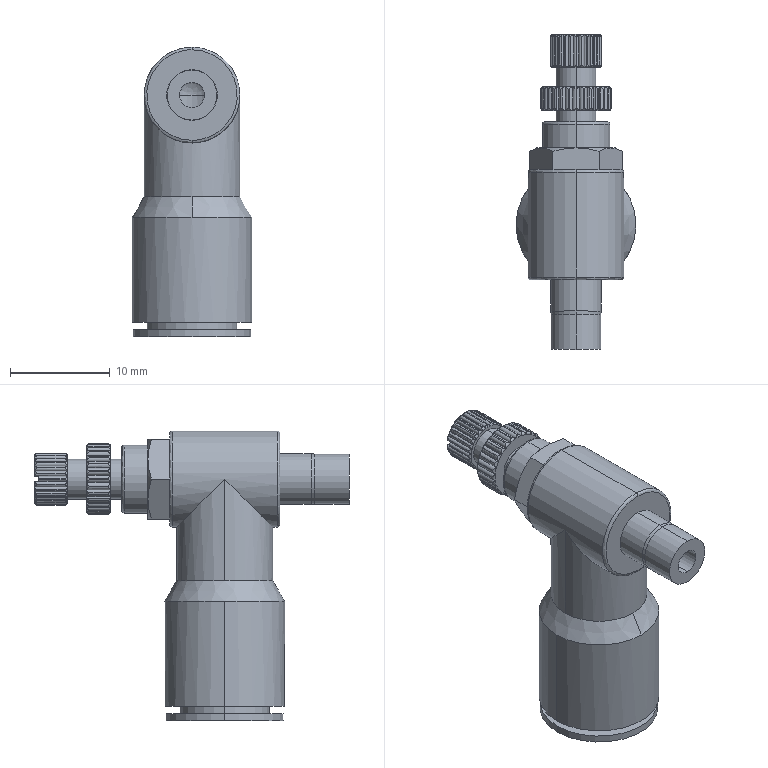Part | SolidWorks | features BaseBody 1 | 1 solid | 445 faces | box 12 x 31.5 x 29 mm | volume 2618 mm3 | cylinder 285 | spline 121 | plane 29 | cone 10 | commonest cylinder face diameters 0.494 x75 0.716 x70 4.724 x28 5.2 x28 6.564 x28 7.04 x28